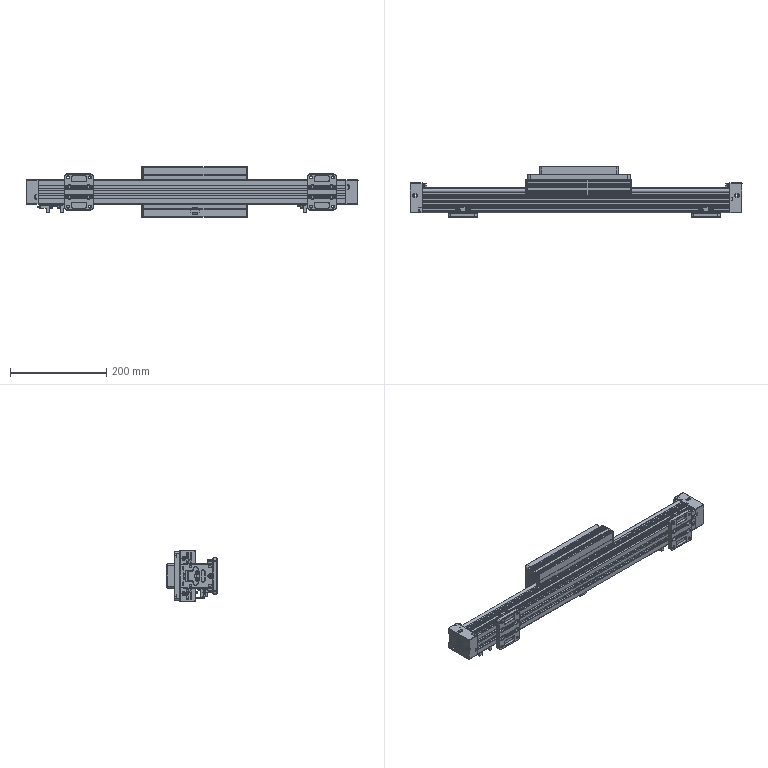Part | SolidWorks | features CompositeCurve 3 | 39 solids | 4493 faces | volume 2196396 mm3 | plane 2446 | cylinder 1261 | cone 556 | spline 182 | torus 48 | commonest cylinder face diameters 0.2 x305 0.4 x116 5.5 x112 5 x90 10 x80 8 x71